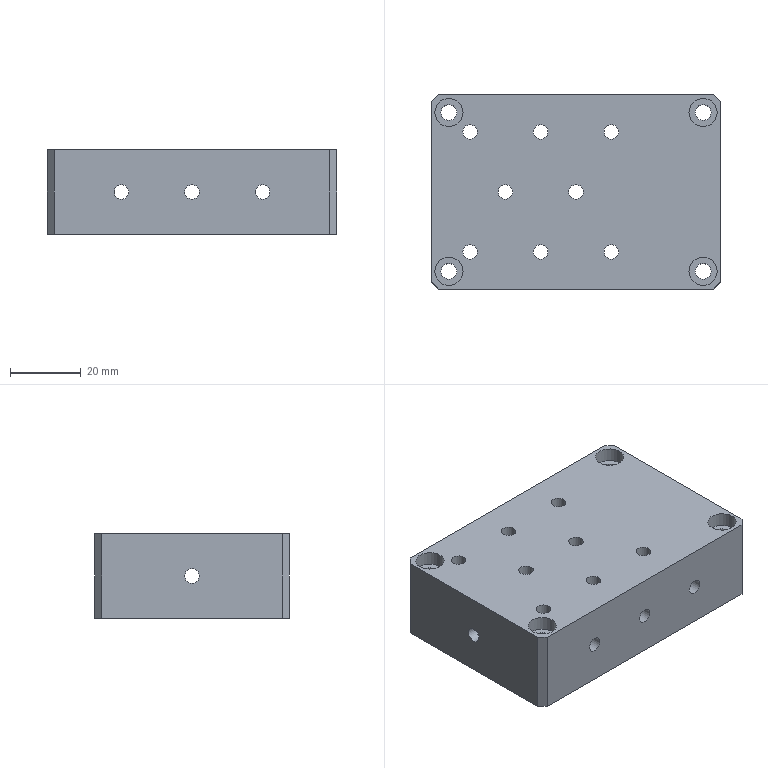NC program | NX | posted with a generic post | part box 82 x 55 x 24 mm
Lines 73 to 908 of 2085:
(ZLEVEL_PROFILE , TOOL : D10)
N126 T15 M6
N128 G54
N130 G17 G0 G90 X-45.662 Y27.593 B0. C0. S9500 M3
N132 G43 Z30. H15
N134 Z1.5
N136 G94 G1 X-44.998 Y28.715 Z1.432 F1000.
N138 X-42.215 Y31.498 Z1.225
N140 X-40.963 Y32.24 Z1.149
N142 X-39.554 Y32.6 Z1.073
N144 X0. Z-1.
N146 X39. F3000.
N148 G2 X42.606 Y31.106 R5.1
N150 G1 X44.606 Y29.106
N152 G2 X46.1 Y25.5 R5.1
N154 G1 Y-25.5
N156 G2 X44.606 Y-29.106 R5.1
N158 G1 X42.606 Y-31.106
N160 G2 X39. Y-32.6 R5.1
N162 G1 X-39.
N164 G2 X-42.606 Y-31.106 R5.1
N166 G1 X-44.606 Y-29.106
N168 G2 X-46.1 Y-25.5 R5.1
N170 G1 Y25.5
N172 G2 X-44.606 Y29.106 R5.1
N174 G1 X-42.606 Y31.106
N176 G2 X-39. Y32.6 R5.1
N178 G1 X0.
N180 X39. Z-1.129
N182 X39.5 Y32.575 Z-1.131
N184 X39.995 Y32.502 Z-1.133
N186 X40.48 Y32.38 Z-1.134
N188 X40.952 Y32.212 Z-1.136
N190 X41.404 Y31.998 Z-1.138
N192 X41.833 Y31.74 Z-1.139
N194 X42.235 Y31.442 Z-1.141
N196 X42.606 Y31.106 Z-1.143
N198 X44.606 Y29.106 Z-1.152
N200 X44.942 Y28.735 Z-1.154
N202 X45.24 Y28.333 Z-1.155
N204 X45.498 Y27.904 Z-1.157
N206 X45.712 Y27.452 Z-1.159
N208 X45.88 Y26.98 Z-1.16
N210 X46.002 Y26.495 Z-1.162
N212 X46.075 Y26. Z-1.164
N214 X46.1 Y25.5 Z-1.165
N216 Y-25.5 Z-1.335
N218 X46.075 Y-26. Z-1.336
N220 X46.002 Y-26.495 Z-1.338
N222 X45.88 Y-26.98 Z-1.34
N224 X45.712 Y-27.452 Z-1.341
N226 X45.498 Y-27.904 Z-1.343
N228 X45.24 Y-28.333 Z-1.345
N230 X44.942 Y-28.735 Z-1.346
N232 X44.606 Y-29.106 Z-1.348
N234 X42.606 Y-31.106 Z-1.357
N236 X42.235 Y-31.442 Z-1.359
N238 X41.833 Y-31.74 Z-1.361
N240 X41.404 Y-31.998 Z-1.362
N242 X40.952 Y-32.212 Z-1.364
N244 X40.48 Y-32.38 Z-1.366
N246 X39.995 Y-32.502 Z-1.367
N248 X39.5 Y-32.575 Z-1.369
N250 X39. Y-32.6 Z-1.371
N252 X-39. Z-1.629
N254 X-39.5 Y-32.575 Z-1.631
N256 X-39.995 Y-32.502 Z-1.633
N258 X-40.48 Y-32.38 Z-1.634
N260 X-40.952 Y-32.212 Z-1.636
N262 X-41.404 Y-31.998 Z-1.638
N264 X-41.833 Y-31.74 Z-1.639
N266 X-42.235 Y-31.442 Z-1.641
N268 X-42.606 Y-31.106 Z-1.643
N270 X-44.606 Y-29.106 Z-1.652
N272 X-44.942 Y-28.735 Z-1.654
N274 X-45.24 Y-28.333 Z-1.655
N276 X-45.498 Y-27.904 Z-1.657
N278 X-45.712 Y-27.452 Z-1.659
N280 X-45.88 Y-26.98 Z-1.66
N282 X-46.002 Y-26.495 Z-1.662
N284 X-46.075 Y-26. Z-1.664
N286 X-46.1 Y-25.5 Z-1.665
N288 Y25.5 Z-1.835
N290 X-46.075 Y26. Z-1.836
N292 X-46.002 Y26.495 Z-1.838
N294 X-45.88 Y26.98 Z-1.84
N296 X-45.712 Y27.452 Z-1.841
N298 X-45.498 Y27.904 Z-1.843
N300 X-45.24 Y28.333 Z-1.845
N302 X-44.942 Y28.735 Z-1.846
N304 X-44.606 Y29.106 Z-1.848
N306 X-42.606 Y31.106 Z-1.857
N308 X-42.235 Y31.442 Z-1.859
N310 X-41.833 Y31.74 Z-1.861
N312 X-41.404 Y31.998 Z-1.862
N314 X-40.952 Y32.212 Z-1.864
N316 X-40.48 Y32.38 Z-1.866
N318 X-39.995 Y32.502 Z-1.867
N320 X-39.5 Y32.575 Z-1.869
N322 X-39. Y32.6 Z-1.871
N324 X0. Z-2.
N326 X39. Z-2.129
N328 X39.5 Y32.575 Z-2.131
N330 X39.995 Y32.502 Z-2.133
N332 X40.48 Y32.38 Z-2.134
N334 X40.952 Y32.212 Z-2.136
N336 X41.404 Y31.998 Z-2.138
N338 X41.833 Y31.74 Z-2.139
N340 X42.235 Y31.442 Z-2.141
N342 X42.606 Y31.106 Z-2.143
N344 X44.606 Y29.106 Z-2.152
N346 X44.942 Y28.735 Z-2.154
N348 X45.24 Y28.333 Z-2.155
N350 X45.498 Y27.904 Z-2.157
N352 X45.712 Y27.452 Z-2.159
N354 X45.88 Y26.98 Z-2.16
N356 X46.002 Y26.495 Z-2.162
N358 X46.075 Y26. Z-2.164
N360 X46.1 Y25.5 Z-2.165
N362 Y-25.5 Z-2.335
N364 X46.075 Y-26. Z-2.336
N366 X46.002 Y-26.495 Z-2.338
N368 X45.88 Y-26.98 Z-2.34
N370 X45.712 Y-27.452 Z-2.341
N372 X45.498 Y-27.904 Z-2.343
N374 X45.24 Y-28.333 Z-2.345
N376 X44.942 Y-28.735 Z-2.346
N378 X44.606 Y-29.106 Z-2.348
N380 X42.606 Y-31.106 Z-2.357
N382 X42.235 Y-31.442 Z-2.359
N384 X41.833 Y-31.74 Z-2.361
N386 X41.404 Y-31.998 Z-2.362
N388 X40.952 Y-32.212 Z-2.364
N390 X40.48 Y-32.38 Z-2.366
N392 X39.995 Y-32.502 Z-2.367
N394 X39.5 Y-32.575 Z-2.369
N396 X39. Y-32.6 Z-2.371
N398 X-39. Z-2.629
N400 X-39.5 Y-32.575 Z-2.631
N402 X-39.995 Y-32.502 Z-2.633
N404 X-40.48 Y-32.38 Z-2.634
N406 X-40.952 Y-32.212 Z-2.636
N408 X-41.404 Y-31.998 Z-2.638
N410 X-41.833 Y-31.74 Z-2.639
N412 X-42.235 Y-31.442 Z-2.641
N414 X-42.606 Y-31.106 Z-2.643
N416 X-44.606 Y-29.106 Z-2.652
N418 X-44.942 Y-28.735 Z-2.654
N420 X-45.24 Y-28.333 Z-2.655
N422 X-45.498 Y-27.904 Z-2.657
N424 X-45.712 Y-27.452 Z-2.659
N426 X-45.88 Y-26.98 Z-2.66
N428 X-46.002 Y-26.495 Z-2.662
N430 X-46.075 Y-26. Z-2.664
N432 X-46.1 Y-25.5 Z-2.665
N434 Y25.5 Z-2.835
N436 X-46.075 Y26. Z-2.836
N438 X-46.002 Y26.495 Z-2.838
N440 X-45.88 Y26.98 Z-2.84
N442 X-45.712 Y27.452 Z-2.841
N444 X-45.498 Y27.904 Z-2.843
N446 X-45.24 Y28.333 Z-2.845
N448 X-44.942 Y28.735 Z-2.846
N450 X-44.606 Y29.106 Z-2.848
N452 X-42.606 Y31.106 Z-2.857
N454 X-42.235 Y31.442 Z-2.859
N456 X-41.833 Y31.74 Z-2.861
N458 X-41.404 Y31.998 Z-2.862
N460 X-40.952 Y32.212 Z-2.864
N462 X-40.48 Y32.38 Z-2.866
N464 X-39.995 Y32.502 Z-2.867
N466 X-39.5 Y32.575 Z-2.869
N468 X-39. Y32.6 Z-2.871
N470 X0. Z-3.
N472 X39. Z-3.129
N474 X39.5 Y32.575 Z-3.131
N476 X39.995 Y32.502 Z-3.133
N478 X40.48 Y32.38 Z-3.134
N480 X40.952 Y32.212 Z-3.136
N482 X41.404 Y31.998 Z-3.138
N484 X41.833 Y31.74 Z-3.139
N486 X42.235 Y31.442 Z-3.141
N488 X42.606 Y31.106 Z-3.143
N490 X44.606 Y29.106 Z-3.152
N492 X44.942 Y28.735 Z-3.154
N494 X45.24 Y28.333 Z-3.155
N496 X45.498 Y27.904 Z-3.157
N498 X45.712 Y27.452 Z-3.159
N500 X45.88 Y26.98 Z-3.16
N502 X46.002 Y26.495 Z-3.162
N504 X46.075 Y26. Z-3.164
N506 X46.1 Y25.5 Z-3.165
N508 Y-25.5 Z-3.335
N510 X46.075 Y-26. Z-3.336
N512 X46.002 Y-26.495 Z-3.338
N514 X45.88 Y-26.98 Z-3.34
N516 X45.712 Y-27.452 Z-3.341
N518 X45.498 Y-27.904 Z-3.343
N520 X45.24 Y-28.333 Z-3.345
N522 X44.942 Y-28.735 Z-3.346
N524 X44.606 Y-29.106 Z-3.348
N526 X42.606 Y-31.106 Z-3.357
N528 X42.235 Y-31.442 Z-3.359
N530 X41.833 Y-31.74 Z-3.361
N532 X41.404 Y-31.998 Z-3.362
N534 X40.952 Y-32.212 Z-3.364
N536 X40.48 Y-32.38 Z-3.366
N538 X39.995 Y-32.502 Z-3.367
N540 X39.5 Y-32.575 Z-3.369
N542 X39. Y-32.6 Z-3.371
N544 X-39. Z-3.629
N546 X-39.5 Y-32.575 Z-3.631
N548 X-39.995 Y-32.502 Z-3.633
N550 X-40.48 Y-32.38 Z-3.634
N552 X-40.952 Y-32.212 Z-3.636
N554 X-41.404 Y-31.998 Z-3.638
N556 X-41.833 Y-31.74 Z-3.639
N558 X-42.235 Y-31.442 Z-3.641
N560 X-42.606 Y-31.106 Z-3.643
N562 X-44.606 Y-29.106 Z-3.652
N564 X-44.942 Y-28.735 Z-3.654
N566 X-45.24 Y-28.333 Z-3.655
N568 X-45.498 Y-27.904 Z-3.657
N570 X-45.712 Y-27.452 Z-3.659
N572 X-45.88 Y-26.98 Z-3.66
N574 X-46.002 Y-26.495 Z-3.662
N576 X-46.075 Y-26. Z-3.664
N578 X-46.1 Y-25.5 Z-3.665
N580 Y25.5 Z-3.835
N582 X-46.075 Y26. Z-3.836
N584 X-46.002 Y26.495 Z-3.838
N586 X-45.88 Y26.98 Z-3.84
N588 X-45.712 Y27.452 Z-3.841
N590 X-45.498 Y27.904 Z-3.843
N592 X-45.24 Y28.333 Z-3.845
N594 X-44.942 Y28.735 Z-3.846
N596 X-44.606 Y29.106 Z-3.848
N598 X-42.606 Y31.106 Z-3.857
N600 X-42.235 Y31.442 Z-3.859
N602 X-41.833 Y31.74 Z-3.861
N604 X-41.404 Y31.998 Z-3.862
N606 X-40.952 Y32.212 Z-3.864
N608 X-40.48 Y32.38 Z-3.866
N610 X-39.995 Y32.502 Z-3.867
N612 X-39.5 Y32.575 Z-3.869
N614 X-39. Y32.6 Z-3.871
N616 X0. Z-4.
N618 X39. Z-4.129
N620 X39.5 Y32.575 Z-4.131
N622 X39.995 Y32.502 Z-4.133
N624 X40.48 Y32.38 Z-4.134
N626 X40.952 Y32.212 Z-4.136
N628 X41.404 Y31.998 Z-4.138
N630 X41.833 Y31.74 Z-4.139
N632 X42.235 Y31.442 Z-4.141
N634 X42.606 Y31.106 Z-4.143
N636 X44.606 Y29.106 Z-4.152
N638 X44.942 Y28.735 Z-4.154
N640 X45.24 Y28.333 Z-4.155
N642 X45.498 Y27.904 Z-4.157
N644 X45.712 Y27.452 Z-4.159
N646 X45.88 Y26.98 Z-4.16
N648 X46.002 Y26.495 Z-4.162
N650 X46.075 Y26. Z-4.164
N652 X46.1 Y25.5 Z-4.165
N654 Y-25.5 Z-4.335
N656 X46.075 Y-26. Z-4.336
N658 X46.002 Y-26.495 Z-4.338
N660 X45.88 Y-26.98 Z-4.34
N662 X45.712 Y-27.452 Z-4.341
N664 X45.498 Y-27.904 Z-4.343
N666 X45.24 Y-28.333 Z-4.345
N668 X44.942 Y-28.735 Z-4.346
N670 X44.606 Y-29.106 Z-4.348
N672 X42.606 Y-31.106 Z-4.357
N674 X42.235 Y-31.442 Z-4.359
N676 X41.833 Y-31.74 Z-4.361
N678 X41.404 Y-31.998 Z-4.362
N680 X40.952 Y-32.212 Z-4.364
N682 X40.48 Y-32.38 Z-4.366
N684 X39.995 Y-32.502 Z-4.367
N686 X39.5 Y-32.575 Z-4.369
N688 X39. Y-32.6 Z-4.371
N690 X-39. Z-4.629
N692 X-39.5 Y-32.575 Z-4.631
N694 X-39.995 Y-32.502 Z-4.633
N696 X-40.48 Y-32.38 Z-4.634
N698 X-40.952 Y-32.212 Z-4.636
N700 X-41.404 Y-31.998 Z-4.638
N702 X-41.833 Y-31.74 Z-4.639
N704 X-42.235 Y-31.442 Z-4.641
N706 X-42.606 Y-31.106 Z-4.643
N708 X-44.606 Y-29.106 Z-4.652
N710 X-44.942 Y-28.735 Z-4.654
N712 X-45.24 Y-28.333 Z-4.655
N714 X-45.498 Y-27.904 Z-4.657
N716 X-45.712 Y-27.452 Z-4.659
N718 X-45.88 Y-26.98 Z-4.66
N720 X-46.002 Y-26.495 Z-4.662
N722 X-46.075 Y-26. Z-4.664
N724 X-46.1 Y-25.5 Z-4.665
N726 Y25.5 Z-4.835
N728 X-46.075 Y26. Z-4.836
N730 X-46.002 Y26.495 Z-4.838
N732 X-45.88 Y26.98 Z-4.84
N734 X-45.712 Y27.452 Z-4.841
N736 X-45.498 Y27.904 Z-4.843
N738 X-45.24 Y28.333 Z-4.845
N740 X-44.942 Y28.735 Z-4.846
N742 X-44.606 Y29.106 Z-4.848
N744 X-42.606 Y31.106 Z-4.857
N746 X-42.235 Y31.442 Z-4.859
N748 X-41.833 Y31.74 Z-4.861
N750 X-41.404 Y31.998 Z-4.862
N752 X-40.952 Y32.212 Z-4.864
N754 X-40.48 Y32.38 Z-4.866
N756 X-39.995 Y32.502 Z-4.867
N758 X-39.5 Y32.575 Z-4.869
N760 X-39. Y32.6 Z-4.871
N762 X0. Z-5.
N764 X39. Z-5.129
N766 X39.5 Y32.575 Z-5.131
N768 X39.995 Y32.502 Z-5.133
N770 X40.48 Y32.38 Z-5.134
N772 X40.952 Y32.212 Z-5.136
N774 X41.404 Y31.998 Z-5.138
N776 X41.833 Y31.74 Z-5.139
N778 X42.235 Y31.442 Z-5.141
N780 X42.606 Y31.106 Z-5.143
N782 X44.606 Y29.106 Z-5.152
N784 X44.942 Y28.735 Z-5.154
N786 X45.24 Y28.333 Z-5.155
N788 X45.498 Y27.904 Z-5.157
N790 X45.712 Y27.452 Z-5.159
N792 X45.88 Y26.98 Z-5.16
N794 X46.002 Y26.495 Z-5.162
N796 X46.075 Y26. Z-5.164
N798 X46.1 Y25.5 Z-5.165
N800 Y-25.5 Z-5.335
N802 X46.075 Y-26. Z-5.336
N804 X46.002 Y-26.495 Z-5.338
N806 X45.88 Y-26.98 Z-5.34
N808 X45.712 Y-27.452 Z-5.341
N810 X45.498 Y-27.904 Z-5.343
N812 X45.24 Y-28.333 Z-5.345
N814 X44.942 Y-28.735 Z-5.346
N816 X44.606 Y-29.106 Z-5.348
N818 X42.606 Y-31.106 Z-5.357
N820 X42.235 Y-31.442 Z-5.359
N822 X41.833 Y-31.74 Z-5.361
N824 X41.404 Y-31.998 Z-5.362
N826 X40.952 Y-32.212 Z-5.364
N828 X40.48 Y-32.38 Z-5.366
N830 X39.995 Y-32.502 Z-5.367
N832 X39.5 Y-32.575 Z-5.369
N834 X39. Y-32.6 Z-5.371
N836 X-39. Z-5.629
N838 X-39.5 Y-32.575 Z-5.631
N840 X-39.995 Y-32.502 Z-5.633
N842 X-40.48 Y-32.38 Z-5.634
N844 X-40.952 Y-32.212 Z-5.636
N846 X-41.404 Y-31.998 Z-5.638
N848 X-41.833 Y-31.74 Z-5.639
N850 X-42.235 Y-31.442 Z-5.641
N852 X-42.606 Y-31.106 Z-5.643
N854 X-44.606 Y-29.106 Z-5.652
N856 X-44.942 Y-28.735 Z-5.654
N858 X-45.24 Y-28.333 Z-5.655
N860 X-45.498 Y-27.904 Z-5.657
N862 X-45.712 Y-27.452 Z-5.659
N864 X-45.88 Y-26.98 Z-5.66
N866 X-46.002 Y-26.495 Z-5.662
N868 X-46.075 Y-26. Z-5.664
N870 X-46.1 Y-25.5 Z-5.665
N872 Y25.5 Z-5.835
N874 X-46.075 Y26. Z-5.836
N876 X-46.002 Y26.495 Z-5.838
N878 X-45.88 Y26.98 Z-5.84
N880 X-45.712 Y27.452 Z-5.841
N882 X-45.498 Y27.904 Z-5.843
N884 X-45.24 Y28.333 Z-5.845
N886 X-44.942 Y28.735 Z-5.846
N888 X-44.606 Y29.106 Z-5.848
N890 X-42.606 Y31.106 Z-5.857
N892 X-42.235 Y31.442 Z-5.859
N894 X-41.833 Y31.74 Z-5.861
N896 X-41.404 Y31.998 Z-5.862
N898 X-40.952 Y32.212 Z-5.864
N900 X-40.48 Y32.38 Z-5.866
N902 X-39.995 Y32.502 Z-5.867
N904 X-39.5 Y32.575 Z-5.869
N906 X-39. Y32.6 Z-5.871
N908 X0. Z-6.
N910 X39. Z-6.129
N912 X39.5 Y32.575 Z-6.131
N914 X39.995 Y32.502 Z-6.133
N916 X40.48 Y32.38 Z-6.134
N918 X40.952 Y32.212 Z-6.136
N920 X41.404 Y31.998 Z-6.138
N922 X41.833 Y31.74 Z-6.139
N924 X42.235 Y31.442 Z-6.141
N926 X42.606 Y31.106 Z-6.143
N928 X44.606 Y29.106 Z-6.152
N930 X44.942 Y28.735 Z-6.154
N932 X45.24 Y28.333 Z-6.155
N934 X45.498 Y27.904 Z-6.157
N936 X45.712 Y27.452 Z-6.159
N938 X45.88 Y26.98 Z-6.16
N940 X46.002 Y26.495 Z-6.162
N942 X46.075 Y26. Z-6.164
N944 X46.1 Y25.5 Z-6.165
N946 Y-25.5 Z-6.335
N948 X46.075 Y-26. Z-6.336
N950 X46.002 Y-26.495 Z-6.338
N952 X45.88 Y-26.98 Z-6.34
N954 X45.712 Y-27.452 Z-6.341
N956 X45.498 Y-27.904 Z-6.343
N958 X45.24 Y-28.333 Z-6.345
N960 X44.942 Y-28.735 Z-6.346
N962 X44.606 Y-29.106 Z-6.348
N964 X42.606 Y-31.106 Z-6.357
N966 X42.235 Y-31.442 Z-6.359
N968 X41.833 Y-31.74 Z-6.361
N970 X41.404 Y-31.998 Z-6.362
N972 X40.952 Y-32.212 Z-6.364
N974 X40.48 Y-32.38 Z-6.366
N976 X39.995 Y-32.502 Z-6.367
N978 X39.5 Y-32.575 Z-6.369
N980 X39. Y-32.6 Z-6.371
N982 X-39. Z-6.629
N984 X-39.5 Y-32.575 Z-6.631
N986 X-39.995 Y-32.502 Z-6.633
N988 X-40.48 Y-32.38 Z-6.634
N990 X-40.952 Y-32.212 Z-6.636
N992 X-41.404 Y-31.998 Z-6.638
N994 X-41.833 Y-31.74 Z-6.639
N996 X-42.235 Y-31.442 Z-6.641
N998 X-42.606 Y-31.106 Z-6.643
N1000 X-44.606 Y-29.106 Z-6.652
N1002 X-44.942 Y-28.735 Z-6.654
N1004 X-45.24 Y-28.333 Z-6.655
N1006 X-45.498 Y-27.904 Z-6.657
N1008 X-45.712 Y-27.452 Z-6.659
N1010 X-45.88 Y-26.98 Z-6.66
N1012 X-46.002 Y-26.495 Z-6.662
N1014 X-46.075 Y-26. Z-6.664
N1016 X-46.1 Y-25.5 Z-6.665
N1018 Y25.5 Z-6.835
N1020 X-46.075 Y26. Z-6.836
N1022 X-46.002 Y26.495 Z-6.838
N1024 X-45.88 Y26.98 Z-6.84
N1026 X-45.712 Y27.452 Z-6.841
N1028 X-45.498 Y27.904 Z-6.843
N1030 X-45.24 Y28.333 Z-6.845
N1032 X-44.942 Y28.735 Z-6.846
N1034 X-44.606 Y29.106 Z-6.848
N1036 X-42.606 Y31.106 Z-6.857
N1038 X-42.235 Y31.442 Z-6.859
N1040 X-41.833 Y31.74 Z-6.861
N1042 X-41.404 Y31.998 Z-6.862
N1044 X-40.952 Y32.212 Z-6.864
N1046 X-40.48 Y32.38 Z-6.866
N1048 X-39.995 Y32.502 Z-6.867
N1050 X-39.5 Y32.575 Z-6.869
N1052 X-39. Y32.6 Z-6.871
N1054 X0. Z-7.
N1056 X39. Z-7.129
N1058 X39.5 Y32.575 Z-7.131
N1060 X39.995 Y32.502 Z-7.133
N1062 X40.48 Y32.38 Z-7.134
N1064 X40.952 Y32.212 Z-7.136
N1066 X41.404 Y31.998 Z-7.138
N1068 X41.833 Y31.74 Z-7.139
N1070 X42.235 Y31.442 Z-7.141
N1072 X42.606 Y31.106 Z-7.143
N1074 X44.606 Y29.106 Z-7.152
N1076 X44.942 Y28.735 Z-7.154
N1078 X45.24 Y28.333 Z-7.155
N1080 X45.498 Y27.904 Z-7.157
N1082 X45.712 Y27.452 Z-7.159
N1084 X45.88 Y26.98 Z-7.16
N1086 X46.002 Y26.495 Z-7.162
N1088 X46.075 Y26. Z-7.164
N1090 X46.1 Y25.5 Z-7.165
N1092 Y-25.5 Z-7.335
N1094 X46.075 Y-26. Z-7.336
N1096 X46.002 Y-26.495 Z-7.338
N1098 X45.88 Y-26.98 Z-7.34
N1100 X45.712 Y-27.452 Z-7.341
N1102 X45.498 Y-27.904 Z-7.343
N1104 X45.24 Y-28.333 Z-7.345
N1106 X44.942 Y-28.735 Z-7.346
N1108 X44.606 Y-29.106 Z-7.348
N1110 X42.606 Y-31.106 Z-7.357
N1112 X42.235 Y-31.442 Z-7.359
N1114 X41.833 Y-31.74 Z-7.361
N1116 X41.404 Y-31.998 Z-7.362
N1118 X40.952 Y-32.212 Z-7.364
N1120 X40.48 Y-32.38 Z-7.366
N1122 X39.995 Y-32.502 Z-7.367
N1124 X39.5 Y-32.575 Z-7.369
N1126 X39. Y-32.6 Z-7.371
N1128 X-39. Z-7.629
N1130 X-39.5 Y-32.575 Z-7.631
N1132 X-39.995 Y-32.502 Z-7.633
N1134 X-40.48 Y-32.38 Z-7.634
N1136 X-40.952 Y-32.212 Z-7.636
N1138 X-41.404 Y-31.998 Z-7.638
N1140 X-41.833 Y-31.74 Z-7.639
N1142 X-42.235 Y-31.442 Z-7.641
N1144 X-42.606 Y-31.106 Z-7.643
N1146 X-44.606 Y-29.106 Z-7.652
N1148 X-44.942 Y-28.735 Z-7.654
N1150 X-45.24 Y-28.333 Z-7.655
N1152 X-45.498 Y-27.904 Z-7.657
N1154 X-45.712 Y-27.452 Z-7.659
N1156 X-45.88 Y-26.98 Z-7.66
N1158 X-46.002 Y-26.495 Z-7.662
N1160 X-46.075 Y-26. Z-7.664
N1162 X-46.1 Y-25.5 Z-7.665
N1164 Y25.5 Z-7.835
N1166 X-46.075 Y26. Z-7.836
N1168 X-46.002 Y26.495 Z-7.838
N1170 X-45.88 Y26.98 Z-7.84
N1172 X-45.712 Y27.452 Z-7.841
N1174 X-45.498 Y27.904 Z-7.843
N1176 X-45.24 Y28.333 Z-7.845
N1178 X-44.942 Y28.735 Z-7.846
N1180 X-44.606 Y29.106 Z-7.848
N1182 X-42.606 Y31.106 Z-7.857
N1184 X-42.235 Y31.442 Z-7.859
N1186 X-41.833 Y31.74 Z-7.861
N1188 X-41.404 Y31.998 Z-7.862
N1190 X-40.952 Y32.212 Z-7.864
N1192 X-40.48 Y32.38 Z-7.866
N1194 X-39.995 Y32.502 Z-7.867
N1196 X-39.5 Y32.575 Z-7.869
N1198 X-39. Y32.6 Z-7.871
N1200 X0. Z-8.
N1202 X39. Z-8.129
N1204 X39.5 Y32.575 Z-8.131
N1206 X39.995 Y32.502 Z-8.133
N1208 X40.48 Y32.38 Z-8.134
N1210 X40.952 Y32.212 Z-8.136
N1212 X41.404 Y31.998 Z-8.138
N1214 X41.833 Y31.74 Z-8.139
N1216 X42.235 Y31.442 Z-8.141
N1218 X42.606 Y31.106 Z-8.143
N1220 X44.606 Y29.106 Z-8.152
N1222 X44.942 Y28.735 Z-8.154
N1224 X45.24 Y28.333 Z-8.155
N1226 X45.498 Y27.904 Z-8.157
N1228 X45.712 Y27.452 Z-8.159
N1230 X45.88 Y26.98 Z-8.16
N1232 X46.002 Y26.495 Z-8.162
N1234 X46.075 Y26. Z-8.164
N1236 X46.1 Y25.5 Z-8.165
N1238 Y-25.5 Z-8.335
N1240 X46.075 Y-26. Z-8.336
N1242 X46.002 Y-26.495 Z-8.338
N1244 X45.88 Y-26.98 Z-8.34
N1246 X45.712 Y-27.452 Z-8.341
N1248 X45.498 Y-27.904 Z-8.343
N1250 X45.24 Y-28.333 Z-8.345
N1252 X44.942 Y-28.735 Z-8.346
N1254 X44.606 Y-29.106 Z-8.348
N1256 X42.606 Y-31.106 Z-8.357
N1258 X42.235 Y-31.442 Z-8.359
N1260 X41.833 Y-31.74 Z-8.361
N1262 X41.404 Y-31.998 Z-8.362
N1264 X40.952 Y-32.212 Z-8.364
N1266 X40.48 Y-32.38 Z-8.366
N1268 X39.995 Y-32.502 Z-8.367
N1270 X39.5 Y-32.575 Z-8.369
N1272 X39. Y-32.6 Z-8.371
N1274 X-39. Z-8.629
N1276 X-39.5 Y-32.575 Z-8.631
N1278 X-39.995 Y-32.502 Z-8.633
N1280 X-40.48 Y-32.38 Z-8.634
N1282 X-40.952 Y-32.212 Z-8.636
N1284 X-41.404 Y-31.998 Z-8.638
N1286 X-41.833 Y-31.74 Z-8.639
N1288 X-42.235 Y-31.442 Z-8.641
N1290 X-42.606 Y-31.106 Z-8.643
N1292 X-44.606 Y-29.106 Z-8.652
N1294 X-44.942 Y-28.735 Z-8.654
N1296 X-45.24 Y-28.333 Z-8.655
N1298 X-45.498 Y-27.904 Z-8.657
N1300 X-45.712 Y-27.452 Z-8.659
N1302 X-45.88 Y-26.98 Z-8.66
N1304 X-46.002 Y-26.495 Z-8.662
N1306 X-46.075 Y-26. Z-8.664
N1308 X-46.1 Y-25.5 Z-8.665
N1310 Y25.5 Z-8.835
N1312 X-46.075 Y26. Z-8.836
N1314 X-46.002 Y26.495 Z-8.838
N1316 X-45.88 Y26.98 Z-8.84
N1318 X-45.712 Y27.452 Z-8.841
N1320 X-45.498 Y27.904 Z-8.843
N1322 X-45.24 Y28.333 Z-8.845
N1324 X-44.942 Y28.735 Z-8.846
N1326 X-44.606 Y29.106 Z-8.848
N1328 X-42.606 Y31.106 Z-8.857
N1330 X-42.235 Y31.442 Z-8.859
N1332 X-41.833 Y31.74 Z-8.861
N1334 X-41.404 Y31.998 Z-8.862
N1336 X-40.952 Y32.212 Z-8.864
N1338 X-40.48 Y32.38 Z-8.866
N1340 X-39.995 Y32.502 Z-8.867
N1342 X-39.5 Y32.575 Z-8.869
N1344 X-39. Y32.6 Z-8.871
N1346 X0. Z-9.
N1348 X39. Z-9.129
N1350 X39.5 Y32.575 Z-9.131
N1352 X39.995 Y32.502 Z-9.133
N1354 X40.48 Y32.38 Z-9.134
N1356 X40.952 Y32.212 Z-9.136
N1358 X41.404 Y31.998 Z-9.138
N1360 X41.833 Y31.74 Z-9.139
N1362 X42.235 Y31.442 Z-9.141
N1364 X42.606 Y31.106 Z-9.143
N1366 X44.606 Y29.106 Z-9.152
N1368 X44.942 Y28.735 Z-9.154
N1370 X45.24 Y28.333 Z-9.155
N1372 X45.498 Y27.904 Z-9.157
N1374 X45.712 Y27.452 Z-9.159
N1376 X45.88 Y26.98 Z-9.16
N1378 X46.002 Y26.495 Z-9.162
N1380 X46.075 Y26. Z-9.164
N1382 X46.1 Y25.5 Z-9.165
N1384 Y-25.5 Z-9.335
N1386 X46.075 Y-26. Z-9.336
N1388 X46.002 Y-26.495 Z-9.338
N1390 X45.88 Y-26.98 Z-9.34
N1392 X45.712 Y-27.452 Z-9.341
N1394 X45.498 Y-27.904 Z-9.343
N1396 X45.24 Y-28.333 Z-9.345
N1398 X44.942 Y-28.735 Z-9.346
N1400 X44.606 Y-29.106 Z-9.348
N1402 X42.606 Y-31.106 Z-9.357
N1404 X42.235 Y-31.442 Z-9.359
N1406 X41.833 Y-31.74 Z-9.361
N1408 X41.404 Y-31.998 Z-9.362
N1410 X40.952 Y-32.212 Z-9.364
N1412 X40.48 Y-32.38 Z-9.366
N1414 X39.995 Y-32.502 Z-9.367
N1416 X39.5 Y-32.575 Z-9.369
N1418 X39. Y-32.6 Z-9.371
N1420 X-39. Z-9.629
N1422 X-39.5 Y-32.575 Z-9.631
N1424 X-39.995 Y-32.502 Z-9.633
N1426 X-40.48 Y-32.38 Z-9.634
N1428 X-40.952 Y-32.212 Z-9.636
N1430 X-41.404 Y-31.998 Z-9.638
N1432 X-41.833 Y-31.74 Z-9.639
N1434 X-42.235 Y-31.442 Z-9.641
N1436 X-42.606 Y-31.106 Z-9.643
N1438 X-44.606 Y-29.106 Z-9.652
N1440 X-44.942 Y-28.735 Z-9.654
N1442 X-45.24 Y-28.333 Z-9.655
N1444 X-45.498 Y-27.904 Z-9.657
N1446 X-45.712 Y-27.452 Z-9.659
N1448 X-45.88 Y-26.98 Z-9.66
N1450 X-46.002 Y-26.495 Z-9.662
N1452 X-46.075 Y-26. Z-9.664
N1454 X-46.1 Y-25.5 Z-9.665
N1456 Y25.5 Z-9.835
N1458 X-46.075 Y26. Z-9.836
N1460 X-46.002 Y26.495 Z-9.838
N1462 X-45.88 Y26.98 Z-9.84
N1464 X-45.712 Y27.452 Z-9.841
N1466 X-45.498 Y27.904 Z-9.843
N1468 X-45.24 Y28.333 Z-9.845
N1470 X-44.942 Y28.735 Z-9.846
N1472 X-44.606 Y29.106 Z-9.848
N1474 X-42.606 Y31.106 Z-9.857
N1476 X-42.235 Y31.442 Z-9.859
N1478 X-41.833 Y31.74 Z-9.861
N1480 X-41.404 Y31.998 Z-9.862
N1482 X-40.952 Y32.212 Z-9.864
N1484 X-40.48 Y32.38 Z-9.866
N1486 X-39.995 Y32.502 Z-9.867
N1488 X-39.5 Y32.575 Z-9.869
N1490 X-39. Y32.6 Z-9.871
N1492 X0. Z-10.
N1494 X39. Z-10.129
N1496 X39.5 Y32.575 Z-10.131
N1498 X39.995 Y32.502 Z-10.133
N1500 X40.48 Y32.38 Z-10.134
N1502 X40.952 Y32.212 Z-10.136
N1504 X41.404 Y31.998 Z-10.138
N1506 X41.833 Y31.74 Z-10.139
N1508 X42.235 Y31.442 Z-10.141
N1510 X42.606 Y31.106 Z-10.143
N1512 X44.606 Y29.106 Z-10.152
N1514 X44.942 Y28.735 Z-10.154
N1516 X45.24 Y28.333 Z-10.155
N1518 X45.498 Y27.904 Z-10.157
N1520 X45.712 Y27.452 Z-10.159
N1522 X45.88 Y26.98 Z-10.16
N1524 X46.002 Y26.495 Z-10.162
N1526 X46.075 Y26. Z-10.164
N1528 X46.1 Y25.5 Z-10.165
N1530 Y-25.5 Z-10.335
N1532 X46.075 Y-26. Z-10.336
N1534 X46.002 Y-26.495 Z-10.338
N1536 X45.88 Y-26.98 Z-10.34
N1538 X45.712 Y-27.452 Z-10.341
N1540 X45.498 Y-27.904 Z-10.343
N1542 X45.24 Y-28.333 Z-10.345
N1544 X44.942 Y-28.735 Z-10.346
N1546 X44.606 Y-29.106 Z-10.348
N1548 X42.606 Y-31.106 Z-10.357
N1550 X42.235 Y-31.442 Z-10.359
N1552 X41.833 Y-31.74 Z-10.361
N1554 X41.404 Y-31.998 Z-10.362
N1556 X40.952 Y-32.212 Z-10.364
N1558 X40.48 Y-32.38 Z-10.366
N1560 X39.995 Y-32.502 Z-10.367
N1562 X39.5 Y-32.575 Z-10.369
N1564 X39. Y-32.6 Z-10.371
N1566 X-39. Z-10.629
N1568 X-39.5 Y-32.575 Z-10.631
N1570 X-39.995 Y-32.502 Z-10.633
N1572 X-40.48 Y-32.38 Z-10.634
N1574 X-40.952 Y-32.212 Z-10.636
N1576 X-41.404 Y-31.998 Z-10.638
N1578 X-41.833 Y-31.74 Z-10.639
N1580 X-42.235 Y-31.442 Z-10.641
N1582 X-42.606 Y-31.106 Z-10.643
N1584 X-44.606 Y-29.106 Z-10.652
N1586 X-44.942 Y-28.735 Z-10.654
N1588 X-45.24 Y-28.333 Z-10.655
N1590 X-45.498 Y-27.904 Z-10.657
N1592 X-45.712 Y-27.452 Z-10.659
N1594 X-45.88 Y-26.98 Z-10.66
N1596 X-46.002 Y-26.495 Z-10.662
N1598 X-46.075 Y-26. Z-10.664
N1600 X-46.1 Y-25.5 Z-10.665
N1602 Y25.5 Z-10.835
N1604 X-46.075 Y26. Z-10.836
N1606 X-46.002 Y26.495 Z-10.838
N1608 X-45.88 Y26.98 Z-10.84
N1610 X-45.712 Y27.452 Z-10.841
N1612 X-45.498 Y27.904 Z-10.843
N1614 X-45.24 Y28.333 Z-10.845
N1616 X-44.942 Y28.735 Z-10.846
N1618 X-44.606 Y29.106 Z-10.848
N1620 X-42.606 Y31.106 Z-10.857
N1622 X-42.235 Y31.442 Z-10.859
N1624 X-41.833 Y31.74 Z-10.861
N1626 X-41.404 Y31.998 Z-10.862
N1628 X-40.952 Y32.212 Z-10.864
N1630 X-40.48 Y32.38 Z-10.866
N1632 X-39.995 Y32.502 Z-10.867
N1634 X-39.5 Y32.575 Z-10.869
N1636 X-39. Y32.6 Z-10.871
N1638 X0. Z-11.
N1640 X39. Z-11.129
N1642 X39.5 Y32.575 Z-11.131
N1644 X39.995 Y32.502 Z-11.133
N1646 X40.48 Y32.38 Z-11.134
N1648 X40.952 Y32.212 Z-11.136
N1650 X41.404 Y31.998 Z-11.138
N1652 X41.833 Y31.74 Z-11.139
N1654 X42.235 Y31.442 Z-11.141
N1656 X42.606 Y31.106 Z-11.143
N1658 X44.606 Y29.106 Z-11.152
N1660 X44.942 Y28.735 Z-11.154
N1662 X45.24 Y28.333 Z-11.155
N1664 X45.498 Y27.904 Z-11.157
N1666 X45.712 Y27.452 Z-11.159
N1668 X45.88 Y26.98 Z-11.16
N1670 X46.002 Y26.495 Z-11.162
N1672 X46.075 Y26. Z-11.164
N1674 X46.1 Y25.5 Z-11.165
N1676 Y-25.5 Z-11.335
N1678 X46.075 Y-26. Z-11.336
N1680 X46.002 Y-26.495 Z-11.338
N1682 X45.88 Y-26.98 Z-11.34
N1684 X45.712 Y-27.452 Z-11.341
N1686 X45.498 Y-27.904 Z-11.343
N1688 X45.24 Y-28.333 Z-11.345
N1690 X44.942 Y-28.735 Z-11.346
N1692 X44.606 Y-29.106 Z-11.348
N1694 X42.606 Y-31.106 Z-11.357
N1696 X42.235 Y-31.442 Z-11.359
N1698 X41.833 Y-31.74 Z-11.361
N1700 X41.404 Y-31.998 Z-11.362
N1702 X40.952 Y-32.212 Z-11.364
N1704 X40.48 Y-32.38 Z-11.366
N1706 X39.995 Y-32.502 Z-11.367
N1708 X39.5 Y-32.575 Z-11.369
N1710 X39. Y-32.6 Z-11.371
N1712 X-39. Z-11.629
N1714 X-39.5 Y-32.575 Z-11.631
N1716 X-39.995 Y-32.502 Z-11.633
N1718 X-40.48 Y-32.38 Z-11.634
N1720 X-40.952 Y-32.212 Z-11.636
N1722 X-41.404 Y-31.998 Z-11.638
N1724 X-41.833 Y-31.74 Z-11.639
N1726 X-42.235 Y-31.442 Z-11.641
N1728 X-42.606 Y-31.106 Z-11.643
N1730 X-44.606 Y-29.106 Z-11.652
N1732 X-44.942 Y-28.735 Z-11.654
N1734 X-45.24 Y-28.333 Z-11.655
N1736 X-45.498 Y-27.904 Z-11.657
N1738 X-45.712 Y-27.452 Z-11.659
N1740 X-45.88 Y-26.98 Z-11.66
N1742 X-46.002 Y-26.495 Z-11.662
N1744 X-46.075 Y-26. Z-11.664
N1746 X-46.1 Y-25.5 Z-11.665
N1748 Y25.5 Z-11.835
N1750 X-46.075 Y26. Z-11.836
N1752 X-46.002 Y26.495 Z-11.838
N1754 X-45.88 Y26.98 Z-11.84
N1756 X-45.712 Y27.452 Z-11.841
N1758 X-45.498 Y27.904 Z-11.843
N1760 X-45.24 Y28.333 Z-11.845
N1762 X-44.942 Y28.735 Z-11.846
N1764 X-44.606 Y29.106 Z-11.848
N1766 X-42.606 Y31.106 Z-11.857
N1768 X-42.235 Y31.442 Z-11.859
N1770 X-41.833 Y31.74 Z-11.861
N1772 X-41.404 Y31.998 Z-11.862
N1774 X-40.952 Y32.212 Z-11.864
N1776 X-40.48 Y32.38 Z-11.866
N1778 X-39.995 Y32.502 Z-11.867
N1780 X-39.5 Y32.575 Z-11.869
N1782 X-39. Y32.6 Z-11.871
N1784 X0. Z-12.
N1786 X39. Z-12.129
N1788 X39.5 Y32.575 Z-12.131
N1790 X39.995 Y32.502 Z-12.133